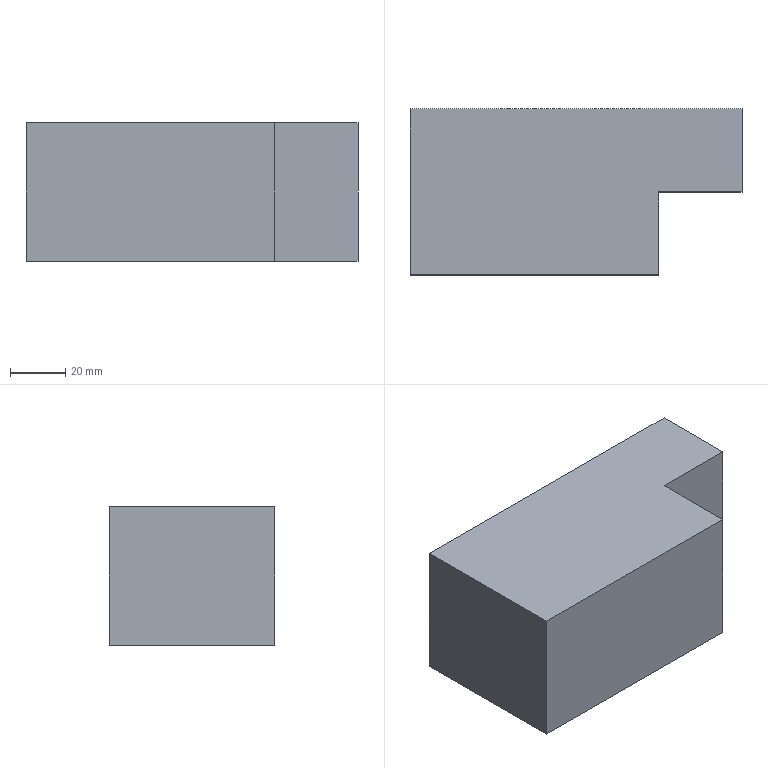Part | NX | features solid 2 | 1 solid | 8 faces | box 120 x 60 x 50 mm | volume 314985 mm3 | plane 8
STEP:
#1=CARTESIAN_POINT('',(-49.99,380.,70.));
#2=VERTEX_POINT('',#1);
#3=CARTESIAN_POINT('',(-80.,380.,70.));
#4=VERTEX_POINT('',#3);
#5=CARTESIAN_POINT('',(-169.99,380.,70.));
#6=DIRECTION('',(-1.,0.,0.));
#7=VECTOR('',#6,1000.);
#8=LINE('',#5,#7);
#9=EDGE_CURVE('',#2,#4,#8,.T.);
#10=ORIENTED_EDGE('',*,*,#9,.T.);
#11=CARTESIAN_POINT('',(-80.,380.,20.));
#12=VERTEX_POINT('',#11);
#13=CARTESIAN_POINT('',(-80.,380.,20.));
#14=DIRECTION('',(0.,0.,1.));
#15=VECTOR('',#14,1000.);
#16=LINE('',#13,#15);
#17=EDGE_CURVE('',#12,#4,#16,.T.);
#18=ORIENTED_EDGE('',*,*,#17,.F.);
#19=CARTESIAN_POINT('',(-49.99,380.,20.));
#20=VERTEX_POINT('',#19);
#21=CARTESIAN_POINT('',(-169.99,380.,20.));
#22=DIRECTION('',(-1.,0.,0.));
#23=VECTOR('',#22,1000.);
#24=LINE('',#21,#23);
#25=EDGE_CURVE('',#20,#12,#24,.T.);
#26=ORIENTED_EDGE('',*,*,#25,.F.);
#27=CARTESIAN_POINT('',(-49.99,380.,70.));
#28=CARTESIAN_POINT('',(-49.99,380.,53.333));
#29=CARTESIAN_POINT('',(-49.99,380.,36.667));
#30=CARTESIAN_POINT('',(-49.99,380.,20.));
#31=B_SPLINE_CURVE_WITH_KNOTS('',3,(#27,#28,#29,#30),.UNSPECIFIED.,.F.,.F.,(4,4),(0.,1.),.UNSPECIFIED.);
#32=EDGE_CURVE('',#20,#2,#31,.F.);
#33=ORIENTED_EDGE('',*,*,#32,.T.);
#34=EDGE_LOOP('',(#10,#18,#26,#33));
#35=FACE_BOUND('',#34,.T.);
#36=CARTESIAN_POINT('',(-169.99,380.,20.));
#37=DIRECTION('',(0.,1.,0.));
#38=DIRECTION('',(-1.,0.,0.));
#39=AXIS2_PLACEMENT_3D('',#36,#37,#38);
#40=PLANE('',#39);
#41=ADVANCED_FACE('',(#35),#40,.F.);
#42=CARTESIAN_POINT('',(-49.99,410.,70.));
#43=VERTEX_POINT('',#42);
#44=CARTESIAN_POINT('',(-49.99,380.,70.));
#45=CARTESIAN_POINT('',(-49.99,390.,70.));
#46=CARTESIAN_POINT('',(-49.99,400.,70.));
#47=CARTESIAN_POINT('',(-49.99,410.,70.));
#48=B_SPLINE_CURVE_WITH_KNOTS('',3,(#44,#45,#46,#47),.UNSPECIFIED.,.F.,.F.,(4,4),(0.,1.),.UNSPECIFIED.);
#49=EDGE_CURVE('',#43,#2,#48,.F.);
#50=ORIENTED_EDGE('',*,*,#49,.T.);
#51=ORIENTED_EDGE('',*,*,#32,.F.);
#52=CARTESIAN_POINT('',(-49.99,410.,20.));
#53=VERTEX_POINT('',#52);
#54=CARTESIAN_POINT('',(-49.99,410.,20.));
#55=CARTESIAN_POINT('',(-49.99,400.,20.));
#56=CARTESIAN_POINT('',(-49.99,390.,20.));
#57=CARTESIAN_POINT('',(-49.99,380.,20.));
#58=B_SPLINE_CURVE_WITH_KNOTS('',3,(#54,#55,#56,#57),.UNSPECIFIED.,.F.,.F.,(4,4),(0.,1.),.UNSPECIFIED.);
#59=EDGE_CURVE('',#53,#20,#58,.T.);
#60=ORIENTED_EDGE('',*,*,#59,.F.);
#61=CARTESIAN_POINT('',(-49.99,410.,70.));
#62=CARTESIAN_POINT('',(-49.99,410.,53.333));
#63=CARTESIAN_POINT('',(-49.99,410.,36.667));
#64=CARTESIAN_POINT('',(-49.99,410.,20.));
#65=B_SPLINE_CURVE_WITH_KNOTS('',3,(#61,#62,#63,#64),.UNSPECIFIED.,.F.,.F.,(4,4),(0.,1.),.UNSPECIFIED.);
#66=EDGE_CURVE('',#53,#43,#65,.F.);
#67=ORIENTED_EDGE('',*,*,#66,.T.);
#68=EDGE_LOOP('',(#50,#51,#60,#67));
#69=FACE_BOUND('',#68,.T.);
#70=CARTESIAN_POINT('',(-49.99,350.,20.));
#71=DIRECTION('',(-1.,0.,0.));
#72=DIRECTION('',(0.,0.,1.));
#73=AXIS2_PLACEMENT_3D('',#70,#71,#72);
#74=PLANE('',#73);
#75=ADVANCED_FACE('',(#69),#74,.F.);
#76=CARTESIAN_POINT('',(-169.99,410.,70.));
#77=VERTEX_POINT('',#76);
#78=CARTESIAN_POINT('',(-49.99,410.,70.));
#79=CARTESIAN_POINT('',(-89.99,410.,70.));
#80=CARTESIAN_POINT('',(-129.99,410.,70.));
#81=CARTESIAN_POINT('',(-169.99,410.,70.));
#82=B_SPLINE_CURVE_WITH_KNOTS('',3,(#78,#79,#80,#81),.UNSPECIFIED.,.F.,.F.,(4,4),(0.,1.),.UNSPECIFIED.);
#83=EDGE_CURVE('',#77,#43,#82,.F.);
#84=ORIENTED_EDGE('',*,*,#83,.T.);
#85=ORIENTED_EDGE('',*,*,#66,.F.);
#86=CARTESIAN_POINT('',(-169.99,410.,20.));
#87=VERTEX_POINT('',#86);
#88=CARTESIAN_POINT('',(-169.99,410.,20.));
#89=CARTESIAN_POINT('',(-129.99,410.,20.));
#90=CARTESIAN_POINT('',(-89.99,410.,20.));
#91=CARTESIAN_POINT('',(-49.99,410.,20.));
#92=B_SPLINE_CURVE_WITH_KNOTS('',3,(#88,#89,#90,#91),.UNSPECIFIED.,.F.,.F.,(4,4),(0.,1.),.UNSPECIFIED.);
#93=EDGE_CURVE('',#87,#53,#92,.T.);
#94=ORIENTED_EDGE('',*,*,#93,.F.);
#95=CARTESIAN_POINT('',(-169.99,410.,70.));
#96=CARTESIAN_POINT('',(-169.99,410.,53.333));
#97=CARTESIAN_POINT('',(-169.99,410.,36.667));
#98=CARTESIAN_POINT('',(-169.99,410.,20.));
#99=B_SPLINE_CURVE_WITH_KNOTS('',3,(#95,#96,#97,#98),.UNSPECIFIED.,.F.,.F.,(4,4),(0.,1.),.UNSPECIFIED.);
#100=EDGE_CURVE('',#87,#77,#99,.F.);
#101=ORIENTED_EDGE('',*,*,#100,.T.);
#102=EDGE_LOOP('',(#84,#85,#94,#101));
#103=FACE_BOUND('',#102,.T.);
#104=CARTESIAN_POINT('',(-169.99,410.,20.));
#105=DIRECTION('',(0.,-1.,0.));
#106=DIRECTION('',(0.,0.,-1.));
#107=AXIS2_PLACEMENT_3D('',#104,#105,#106);
#108=PLANE('',#107);
#109=ADVANCED_FACE('',(#103),#108,.F.);
#110=CARTESIAN_POINT('',(-169.99,350.,70.));
#111=VERTEX_POINT('',#110);
#112=CARTESIAN_POINT('',(-169.99,410.,70.));
#113=CARTESIAN_POINT('',(-169.99,390.,70.));
#114=CARTESIAN_POINT('',(-169.99,370.,70.));
#115=CARTESIAN_POINT('',(-169.99,350.,70.));
#116=B_SPLINE_CURVE_WITH_KNOTS('',3,(#112,#113,#114,#115),.UNSPECIFIED.,.F.,.F.,(4,4),(0.,1.),.UNSPECIFIED.);
#117=EDGE_CURVE('',#77,#111,#116,.T.);
#118=ORIENTED_EDGE('',*,*,#117,.F.);
#119=ORIENTED_EDGE('',*,*,#100,.F.);
#120=CARTESIAN_POINT('',(-169.99,350.,20.));
#121=VERTEX_POINT('',#120);
#122=CARTESIAN_POINT('',(-169.99,350.,20.));
#123=CARTESIAN_POINT('',(-169.99,370.,20.));
#124=CARTESIAN_POINT('',(-169.99,390.,20.));
#125=CARTESIAN_POINT('',(-169.99,410.,20.));
#126=B_SPLINE_CURVE_WITH_KNOTS('',3,(#122,#123,#124,#125),.UNSPECIFIED.,.F.,.F.,(4,4),(0.,1.),.UNSPECIFIED.);
#127=EDGE_CURVE('',#87,#121,#126,.F.);
#128=ORIENTED_EDGE('',*,*,#127,.T.);
#129=CARTESIAN_POINT('',(-169.99,350.,70.));
#130=CARTESIAN_POINT('',(-169.99,350.,53.333));
#131=CARTESIAN_POINT('',(-169.99,350.,36.667));
#132=CARTESIAN_POINT('',(-169.99,350.,20.));
#133=B_SPLINE_CURVE_WITH_KNOTS('',3,(#129,#130,#131,#132),.UNSPECIFIED.,.F.,.F.,(4,4),(0.,1.),.UNSPECIFIED.);
#134=EDGE_CURVE('',#121,#111,#133,.F.);
#135=ORIENTED_EDGE('',*,*,#134,.T.);
#136=EDGE_LOOP('',(#118,#119,#128,#135));
#137=FACE_BOUND('',#136,.T.);
#138=CARTESIAN_POINT('',(-169.99,350.,20.));
#139=DIRECTION('',(-1.,0.,0.));
#140=DIRECTION('',(0.,0.,1.));
#141=AXIS2_PLACEMENT_3D('',#138,#139,#140);
#142=PLANE('',#141);
#143=ADVANCED_FACE('',(#137),#142,.T.);
#144=CARTESIAN_POINT('',(-80.,350.,70.));
#145=VERTEX_POINT('',#144);
#146=CARTESIAN_POINT('',(-169.99,350.,70.));
#147=CARTESIAN_POINT('',(-139.993,350.,70.));
#148=CARTESIAN_POINT('',(-109.997,350.,70.));
#149=CARTESIAN_POINT('',(-80.,350.,70.));
#150=B_SPLINE_CURVE_WITH_KNOTS('',3,(#146,#147,#148,#149),.UNSPECIFIED.,.F.,.F.,(4,4),(0.,1.),.UNSPECIFIED.);
#151=EDGE_CURVE('',#111,#145,#150,.T.);
#152=ORIENTED_EDGE('',*,*,#151,.F.);
#153=ORIENTED_EDGE('',*,*,#134,.F.);
#154=CARTESIAN_POINT('',(-80.,350.,20.));
#155=VERTEX_POINT('',#154);
#156=CARTESIAN_POINT('',(-80.,350.,20.));
#157=CARTESIAN_POINT('',(-109.997,350.,20.));
#158=CARTESIAN_POINT('',(-139.993,350.,20.));
#159=CARTESIAN_POINT('',(-169.99,350.,20.));
#160=B_SPLINE_CURVE_WITH_KNOTS('',3,(#156,#157,#158,#159),.UNSPECIFIED.,.F.,.F.,(4,4),(0.,1.),.UNSPECIFIED.);
#161=EDGE_CURVE('',#121,#155,#160,.F.);
#162=ORIENTED_EDGE('',*,*,#161,.T.);
#163=CARTESIAN_POINT('',(-80.,350.,70.));
#164=CARTESIAN_POINT('',(-80.,350.,53.333));
#165=CARTESIAN_POINT('',(-80.,350.,36.667));
#166=CARTESIAN_POINT('',(-80.,350.,20.));
#167=B_SPLINE_CURVE_WITH_KNOTS('',3,(#163,#164,#165,#166),.UNSPECIFIED.,.F.,.F.,(4,4),(0.,1.),.UNSPECIFIED.);
#168=EDGE_CURVE('',#155,#145,#167,.F.);
#169=ORIENTED_EDGE('',*,*,#168,.T.);
#170=EDGE_LOOP('',(#152,#153,#162,#169));
#171=FACE_BOUND('',#170,.T.);
#172=CARTESIAN_POINT('',(-169.99,350.,20.));
#173=DIRECTION('',(0.,-1.,0.));
#174=DIRECTION('',(0.,0.,-1.));
#175=AXIS2_PLACEMENT_3D('',#172,#173,#174);
#176=PLANE('',#175);
#177=ADVANCED_FACE('',(#171),#176,.T.);
#178=CARTESIAN_POINT('',(-80.,365.,70.));
#179=DIRECTION('',(0.,-1.,0.));
#180=VECTOR('',#179,1000.);
#181=LINE('',#178,#180);
#182=EDGE_CURVE('',#4,#145,#181,.T.);
#183=ORIENTED_EDGE('',*,*,#182,.T.);
#184=ORIENTED_EDGE('',*,*,#168,.F.);
#185=CARTESIAN_POINT('',(-80.,365.,20.));
#186=DIRECTION('',(0.,-1.,0.));
#187=VECTOR('',#186,1000.);
#188=LINE('',#185,#187);
#189=EDGE_CURVE('',#12,#155,#188,.T.);
#190=ORIENTED_EDGE('',*,*,#189,.F.);
#191=ORIENTED_EDGE('',*,*,#17,.T.);
#192=EDGE_LOOP('',(#183,#184,#190,#191));
#193=FACE_BOUND('',#192,.T.);
#194=CARTESIAN_POINT('',(-80.,365.,20.));
#195=DIRECTION('',(-1.,0.,0.));
#196=DIRECTION('',(0.,-1.,0.));
#197=AXIS2_PLACEMENT_3D('',#194,#195,#196);
#198=PLANE('',#197);
#199=ADVANCED_FACE('',(#193),#198,.F.);
#200=ORIENTED_EDGE('',*,*,#25,.T.);
#201=ORIENTED_EDGE('',*,*,#189,.T.);
#202=ORIENTED_EDGE('',*,*,#161,.F.);
#203=ORIENTED_EDGE('',*,*,#127,.F.);
#204=ORIENTED_EDGE('',*,*,#93,.T.);
#205=ORIENTED_EDGE('',*,*,#59,.T.);
#206=EDGE_LOOP('',(#200,#201,#202,#203,#204,#205));
#207=FACE_BOUND('',#206,.T.);
#208=CARTESIAN_POINT('',(-169.99,350.,20.));
#209=DIRECTION('',(0.,0.,1.));
#210=DIRECTION('',(1.,0.,0.));
#211=AXIS2_PLACEMENT_3D('',#208,#209,#210);
#212=PLANE('',#211);
#213=ADVANCED_FACE('',(#207),#212,.F.);
#214=ORIENTED_EDGE('',*,*,#9,.F.);
#215=ORIENTED_EDGE('',*,*,#49,.F.);
#216=ORIENTED_EDGE('',*,*,#83,.F.);
#217=ORIENTED_EDGE('',*,*,#117,.T.);
#218=ORIENTED_EDGE('',*,*,#151,.T.);
#219=ORIENTED_EDGE('',*,*,#182,.F.);
#220=EDGE_LOOP('',(#214,#215,#216,#217,#218,#219));
#221=FACE_BOUND('',#220,.T.);
#222=CARTESIAN_POINT('',(-169.99,350.,70.));
#223=DIRECTION('',(0.,0.,1.));
#224=DIRECTION('',(1.,0.,0.));
#225=AXIS2_PLACEMENT_3D('',#222,#223,#224);
#226=PLANE('',#225);
#227=ADVANCED_FACE('',(#221),#226,.T.);
#228=CLOSED_SHELL('',(#41,#75,#109,#143,#177,#199,#213,#227));
#229=MANIFOLD_SOLID_BREP('',#228);
#230=(LENGTH_UNIT()NAMED_UNIT(*)SI_UNIT(.MILLI.,.METRE.));
#231=UNCERTAINTY_MEASURE_WITH_UNIT(LENGTH_MEASURE(0.0508),#230,'','');
#232=(NAMED_UNIT(*)PLANE_ANGLE_UNIT()SI_UNIT($,.RADIAN.));
#233=(NAMED_UNIT(*)SI_UNIT($,.STERADIAN.)SOLID_ANGLE_UNIT());
#234=(GEOMETRIC_REPRESENTATION_CONTEXT(3)GLOBAL_UNCERTAINTY_ASSIGNED_CONTEXT((#231))GLOBAL_UNIT_ASSIGNED_CONTEXT((#230,#232,#233))REPRESENTATION_CONTEXT('',''));
#235=ADVANCED_BREP_SHAPE_REPRESENTATION('',(#229),#234);